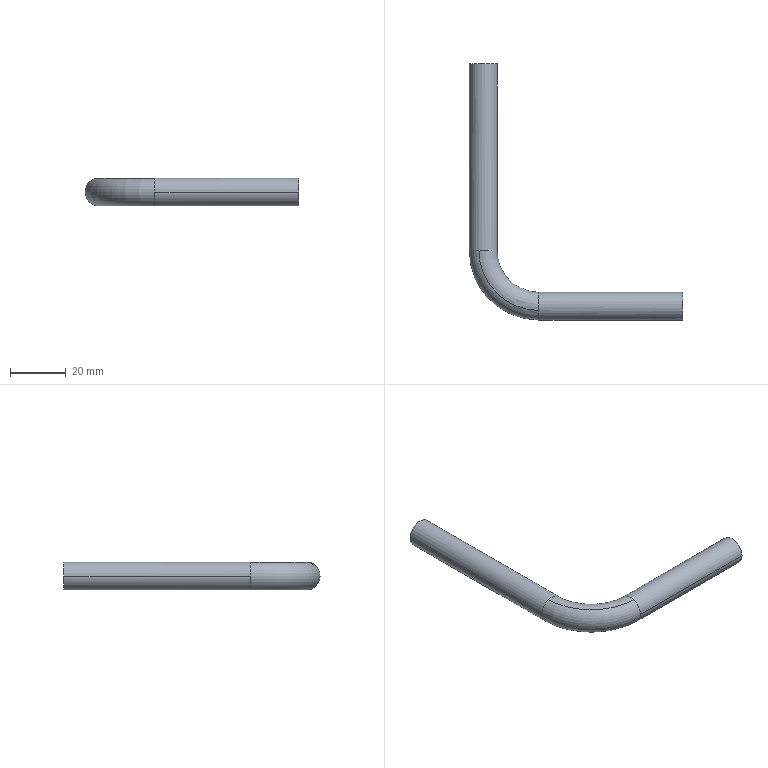Part | 1 solid | 8 faces | box 76.634 x 92 x 10 mm | volume 11785 mm3 | cylinder 4 | plane 2 | torus 2 | commonest cylinder face diameters 10 x4
STEP:
#1=CARTESIAN_POINT('',(0.,0.,0.));
#2=DIRECTION('',(0.,0.,1.));
#3=DIRECTION('',(1.,0.,0.));
#4=AXIS2_PLACEMENT_3D('',#1,#2,#3);
#5=CARTESIAN_POINT('',(-70.758,421.551,-68.051));
#6=VERTEX_POINT('',#5);
#7=CARTESIAN_POINT('',(-70.758,488.551,-68.051));
#8=VERTEX_POINT('',#7);
#9=CARTESIAN_POINT('',(-70.758,421.551,-68.051));
#10=DIRECTION('',(0.,1.,0.));
#11=VECTOR('',#10,1.);
#12=LINE('',#9,#11);
#13=CARTESIAN_POINT('',(-75.758,421.551,-68.051));
#14=DIRECTION('',(0.,1.,0.));
#15=DIRECTION('',(0.,0.,1.));
#16=AXIS2_PLACEMENT_3D('',#13,#14,#15);
#17=CYLINDRICAL_SURFACE('',#16,5.);
#18=CARTESIAN_POINT('',(1.571,0.));
#19=DIRECTION('',(0.,1.));
#20=VECTOR('',#19,1.);
#21=LINE('',#18,#20);
#22=(GEOMETRIC_REPRESENTATION_CONTEXT(2)PARAMETRIC_REPRESENTATION_CONTEXT()REPRESENTATION_CONTEXT('',''));
#23=DEFINITIONAL_REPRESENTATION('',(#21),#22);
#24=PCURVE('',#17,#23);
#25=CARTESIAN_POINT('',(-75.758,421.551,-68.051));
#26=DIRECTION('',(0.,1.,0.));
#27=DIRECTION('',(0.,0.,-1.));
#28=AXIS2_PLACEMENT_3D('',#25,#26,#27);
#29=CYLINDRICAL_SURFACE('',#28,5.);
#30=CARTESIAN_POINT('',(4.712,0.));
#31=DIRECTION('',(0.,1.));
#32=VECTOR('',#31,1.);
#33=LINE('',#30,#32);
#34=(GEOMETRIC_REPRESENTATION_CONTEXT(2)PARAMETRIC_REPRESENTATION_CONTEXT()REPRESENTATION_CONTEXT('',''));
#35=DEFINITIONAL_REPRESENTATION('',(#33),#34);
#36=PCURVE('',#29,#35);
#37=SURFACE_CURVE('',#12,(#24,#36),.PCURVE_S1.);
#38=EDGE_CURVE('',#6,#8,#37,.T.);
#39=ORIENTED_EDGE('',*,*,#38,.F.);
#40=CARTESIAN_POINT('',(-74.213,421.551,-72.807));
#41=VERTEX_POINT('',#40);
#42=CARTESIAN_POINT('',(-75.758,421.551,-68.051));
#43=DIRECTION('',(0.,1.,0.));
#44=DIRECTION('',(-1.,0.,0.));
#45=AXIS2_PLACEMENT_3D('',#42,#43,#44);
#46=CIRCLE('',#45,5.);
#47=CARTESIAN_POINT('',(-1.571,0.));
#48=DIRECTION('',(1.,0.));
#49=VECTOR('',#48,1.);
#50=LINE('',#47,#49);
#51=(GEOMETRIC_REPRESENTATION_CONTEXT(2)PARAMETRIC_REPRESENTATION_CONTEXT()REPRESENTATION_CONTEXT('',''));
#52=DEFINITIONAL_REPRESENTATION('',(#50),#51);
#53=PCURVE('',#17,#52);
#54=CARTESIAN_POINT('',(-55.758,421.551,-68.051));
#55=DIRECTION('',(0.,0.,1.));
#56=DIRECTION('',(0.7071,0.7071,0.));
#57=AXIS2_PLACEMENT_3D('',#54,#55,#56);
#58=TOROIDAL_SURFACE('',#57,20.,5.);
#59=CARTESIAN_POINT('',(2.356,0.));
#60=DIRECTION('',(0.,1.));
#61=VECTOR('',#60,1.);
#62=LINE('',#59,#61);
#63=(GEOMETRIC_REPRESENTATION_CONTEXT(2)PARAMETRIC_REPRESENTATION_CONTEXT()REPRESENTATION_CONTEXT('',''));
#64=DEFINITIONAL_REPRESENTATION('',(#62),#63);
#65=PCURVE('',#58,#64);
#66=SURFACE_CURVE('',#46,(#53,#65),.PCURVE_S1.);
#67=EDGE_CURVE('',#6,#41,#66,.T.);
#68=ORIENTED_EDGE('',*,*,#67,.T.);
#69=CARTESIAN_POINT('',(-80.758,421.551,-68.051));
#70=VERTEX_POINT('',#69);
#71=CARTESIAN_POINT('',(-75.758,421.551,-68.051));
#72=DIRECTION('',(0.,1.,0.));
#73=DIRECTION('',(-1.,0.,0.));
#74=AXIS2_PLACEMENT_3D('',#71,#72,#73);
#75=CIRCLE('',#74,5.);
#76=CARTESIAN_POINT('',(-1.571,0.));
#77=DIRECTION('',(1.,0.));
#78=VECTOR('',#77,1.);
#79=LINE('',#76,#78);
#80=(GEOMETRIC_REPRESENTATION_CONTEXT(2)PARAMETRIC_REPRESENTATION_CONTEXT()REPRESENTATION_CONTEXT('',''));
#81=DEFINITIONAL_REPRESENTATION('',(#79),#80);
#82=PCURVE('',#17,#81);
#83=CARTESIAN_POINT('',(-55.758,421.551,-68.051));
#84=DIRECTION('',(0.,0.,1.));
#85=DIRECTION('',(0.7071,0.7071,0.));
#86=AXIS2_PLACEMENT_3D('',#83,#84,#85);
#87=TOROIDAL_SURFACE('',#86,20.,5.);
#88=CARTESIAN_POINT('',(2.356,0.));
#89=DIRECTION('',(0.,1.));
#90=VECTOR('',#89,1.);
#91=LINE('',#88,#90);
#92=(GEOMETRIC_REPRESENTATION_CONTEXT(2)PARAMETRIC_REPRESENTATION_CONTEXT()REPRESENTATION_CONTEXT('',''));
#93=DEFINITIONAL_REPRESENTATION('',(#91),#92);
#94=PCURVE('',#87,#93);
#95=SURFACE_CURVE('',#75,(#82,#94),.PCURVE_S1.);
#96=EDGE_CURVE('',#41,#70,#95,.T.);
#97=ORIENTED_EDGE('',*,*,#96,.T.);
#98=CARTESIAN_POINT('',(-80.758,488.551,-68.051));
#99=VERTEX_POINT('',#98);
#100=CARTESIAN_POINT('',(-80.758,421.551,-68.051));
#101=DIRECTION('',(0.,1.,0.));
#102=VECTOR('',#101,1.);
#103=LINE('',#100,#102);
#104=CARTESIAN_POINT('',(4.712,0.));
#105=DIRECTION('',(0.,1.));
#106=VECTOR('',#105,1.);
#107=LINE('',#104,#106);
#108=(GEOMETRIC_REPRESENTATION_CONTEXT(2)PARAMETRIC_REPRESENTATION_CONTEXT()REPRESENTATION_CONTEXT('',''));
#109=DEFINITIONAL_REPRESENTATION('',(#107),#108);
#110=PCURVE('',#17,#109);
#111=CARTESIAN_POINT('',(1.571,0.));
#112=DIRECTION('',(0.,1.));
#113=VECTOR('',#112,1.);
#114=LINE('',#111,#113);
#115=(GEOMETRIC_REPRESENTATION_CONTEXT(2)PARAMETRIC_REPRESENTATION_CONTEXT()REPRESENTATION_CONTEXT('',''));
#116=DEFINITIONAL_REPRESENTATION('',(#114),#115);
#117=PCURVE('',#29,#116);
#118=SURFACE_CURVE('',#103,(#110,#117),.PCURVE_S1.);
#119=EDGE_CURVE('',#70,#99,#118,.T.);
#120=ORIENTED_EDGE('',*,*,#119,.T.);
#121=CARTESIAN_POINT('',(-75.758,488.551,-68.051));
#122=DIRECTION('',(0.,1.,0.));
#123=DIRECTION('',(-1.,0.,0.));
#124=AXIS2_PLACEMENT_3D('',#121,#122,#123);
#125=CIRCLE('',#124,5.);
#126=CARTESIAN_POINT('',(-1.571,67.));
#127=DIRECTION('',(1.,0.));
#128=VECTOR('',#127,1.);
#129=LINE('',#126,#128);
#130=(GEOMETRIC_REPRESENTATION_CONTEXT(2)PARAMETRIC_REPRESENTATION_CONTEXT()REPRESENTATION_CONTEXT('',''));
#131=DEFINITIONAL_REPRESENTATION('',(#129),#130);
#132=PCURVE('',#17,#131);
#133=CARTESIAN_POINT('',(-75.758,488.551,-68.051));
#134=DIRECTION('',(0.,1.,0.));
#135=DIRECTION('',(-1.,0.,0.));
#136=AXIS2_PLACEMENT_3D('',#133,#134,#135);
#137=PLANE('',#136);
#138=CARTESIAN_POINT('',(0.,0.));
#139=DIRECTION('',(1.,0.));
#140=AXIS2_PLACEMENT_2D('',#138,#139);
#141=CIRCLE('',#140,5.);
#142=(GEOMETRIC_REPRESENTATION_CONTEXT(2)PARAMETRIC_REPRESENTATION_CONTEXT()REPRESENTATION_CONTEXT('',''));
#143=DEFINITIONAL_REPRESENTATION('',(#141),#142);
#144=PCURVE('',#137,#143);
#145=SURFACE_CURVE('',#125,(#132,#144),.PCURVE_S1.);
#146=EDGE_CURVE('',#8,#99,#145,.T.);
#147=ORIENTED_EDGE('',*,*,#146,.F.);
#148=EDGE_LOOP('',(#39,#68,#97,#120,#147));
#149=FACE_BOUND('',#148,.T.);
#150=ADVANCED_FACE('',(#149),#17,.T.);
#151=CARTESIAN_POINT('',(-75.758,488.551,-68.051));
#152=DIRECTION('',(0.,1.,0.));
#153=DIRECTION('',(-1.,0.,0.));
#154=AXIS2_PLACEMENT_3D('',#151,#152,#153);
#155=CIRCLE('',#154,5.);
#156=CARTESIAN_POINT('',(0.,0.));
#157=DIRECTION('',(1.,0.));
#158=AXIS2_PLACEMENT_2D('',#156,#157);
#159=CIRCLE('',#158,5.);
#160=(GEOMETRIC_REPRESENTATION_CONTEXT(2)PARAMETRIC_REPRESENTATION_CONTEXT()REPRESENTATION_CONTEXT('',''));
#161=DEFINITIONAL_REPRESENTATION('',(#159),#160);
#162=PCURVE('',#137,#161);
#163=CARTESIAN_POINT('',(1.571,67.));
#164=DIRECTION('',(1.,0.));
#165=VECTOR('',#164,1.);
#166=LINE('',#163,#165);
#167=(GEOMETRIC_REPRESENTATION_CONTEXT(2)PARAMETRIC_REPRESENTATION_CONTEXT()REPRESENTATION_CONTEXT('',''));
#168=DEFINITIONAL_REPRESENTATION('',(#166),#167);
#169=PCURVE('',#29,#168);
#170=SURFACE_CURVE('',#155,(#162,#169),.PCURVE_S1.);
#171=EDGE_CURVE('',#99,#8,#170,.T.);
#172=ORIENTED_EDGE('',*,*,#171,.T.);
#173=ORIENTED_EDGE('',*,*,#146,.T.);
#174=EDGE_LOOP('',(#172,#173));
#175=FACE_BOUND('',#174,.T.);
#176=ADVANCED_FACE('',(#175),#137,.T.);
#177=CARTESIAN_POINT('',(-55.758,403.096,-72.807));
#178=VERTEX_POINT('',#177);
#179=CARTESIAN_POINT('',(-55.758,421.551,-72.807));
#180=DIRECTION('',(0.,0.,1.));
#181=DIRECTION('',(-1.,0.,0.));
#182=AXIS2_PLACEMENT_3D('',#179,#180,#181);
#183=CIRCLE('',#182,18.455);
#184=CARTESIAN_POINT('',(2.356,4.398));
#185=DIRECTION('',(1.,0.));
#186=VECTOR('',#185,1.);
#187=LINE('',#184,#186);
#188=(GEOMETRIC_REPRESENTATION_CONTEXT(2)PARAMETRIC_REPRESENTATION_CONTEXT()REPRESENTATION_CONTEXT('',''));
#189=DEFINITIONAL_REPRESENTATION('',(#187),#188);
#190=PCURVE('',#58,#189);
#191=CARTESIAN_POINT('',(2.356,4.398));
#192=DIRECTION('',(1.,0.));
#193=VECTOR('',#192,1.);
#194=LINE('',#191,#193);
#195=(GEOMETRIC_REPRESENTATION_CONTEXT(2)PARAMETRIC_REPRESENTATION_CONTEXT()REPRESENTATION_CONTEXT('',''));
#196=DEFINITIONAL_REPRESENTATION('',(#194),#195);
#197=PCURVE('',#87,#196);
#198=SURFACE_CURVE('',#183,(#190,#197),.PCURVE_S1.);
#199=EDGE_CURVE('',#41,#178,#198,.T.);
#200=ORIENTED_EDGE('',*,*,#199,.F.);
#201=ORIENTED_EDGE('',*,*,#67,.F.);
#202=CARTESIAN_POINT('',(-77.304,421.551,-63.296));
#203=VERTEX_POINT('',#202);
#204=CARTESIAN_POINT('',(-75.758,421.551,-68.051));
#205=DIRECTION('',(0.,1.,0.));
#206=DIRECTION('',(-1.,0.,0.));
#207=AXIS2_PLACEMENT_3D('',#204,#205,#206);
#208=CIRCLE('',#207,5.);
#209=CARTESIAN_POINT('',(2.356,0.));
#210=DIRECTION('',(0.,1.));
#211=VECTOR('',#210,1.);
#212=LINE('',#209,#211);
#213=(GEOMETRIC_REPRESENTATION_CONTEXT(2)PARAMETRIC_REPRESENTATION_CONTEXT()REPRESENTATION_CONTEXT('',''));
#214=DEFINITIONAL_REPRESENTATION('',(#212),#213);
#215=PCURVE('',#58,#214);
#216=CARTESIAN_POINT('',(1.571,0.));
#217=DIRECTION('',(1.,0.));
#218=VECTOR('',#217,1.);
#219=LINE('',#216,#218);
#220=(GEOMETRIC_REPRESENTATION_CONTEXT(2)PARAMETRIC_REPRESENTATION_CONTEXT()REPRESENTATION_CONTEXT('',''));
#221=DEFINITIONAL_REPRESENTATION('',(#219),#220);
#222=PCURVE('',#29,#221);
#223=SURFACE_CURVE('',#208,(#215,#222),.PCURVE_S1.);
#224=EDGE_CURVE('',#203,#6,#223,.T.);
#225=ORIENTED_EDGE('',*,*,#224,.F.);
#226=CARTESIAN_POINT('',(-55.758,400.006,-63.296));
#227=VERTEX_POINT('',#226);
#228=CARTESIAN_POINT('',(-55.758,421.551,-63.296));
#229=DIRECTION('',(0.,0.,1.));
#230=DIRECTION('',(-1.,0.,0.));
#231=AXIS2_PLACEMENT_3D('',#228,#229,#230);
#232=CIRCLE('',#231,21.545);
#233=CARTESIAN_POINT('',(2.356,1.257));
#234=DIRECTION('',(1.,0.));
#235=VECTOR('',#234,1.);
#236=LINE('',#233,#235);
#237=(GEOMETRIC_REPRESENTATION_CONTEXT(2)PARAMETRIC_REPRESENTATION_CONTEXT()REPRESENTATION_CONTEXT('',''));
#238=DEFINITIONAL_REPRESENTATION('',(#236),#237);
#239=PCURVE('',#58,#238);
#240=CARTESIAN_POINT('',(2.356,7.54));
#241=DIRECTION('',(1.,0.));
#242=VECTOR('',#241,1.);
#243=LINE('',#240,#242);
#244=(GEOMETRIC_REPRESENTATION_CONTEXT(2)PARAMETRIC_REPRESENTATION_CONTEXT()REPRESENTATION_CONTEXT('',''));
#245=DEFINITIONAL_REPRESENTATION('',(#243),#244);
#246=PCURVE('',#87,#245);
#247=SURFACE_CURVE('',#232,(#239,#246),.PCURVE_S1.);
#248=EDGE_CURVE('',#203,#227,#247,.T.);
#249=ORIENTED_EDGE('',*,*,#248,.T.);
#250=CARTESIAN_POINT('',(-55.758,406.551,-68.051));
#251=VERTEX_POINT('',#250);
#252=CARTESIAN_POINT('',(-55.758,401.551,-68.051));
#253=DIRECTION('',(-1.,0.,0.));
#254=DIRECTION('',(0.,-1.,0.));
#255=AXIS2_PLACEMENT_3D('',#252,#253,#254);
#256=CIRCLE('',#255,5.);
#257=CARTESIAN_POINT('',(3.927,0.));
#258=DIRECTION('',(0.,1.));
#259=VECTOR('',#258,1.);
#260=LINE('',#257,#259);
#261=(GEOMETRIC_REPRESENTATION_CONTEXT(2)PARAMETRIC_REPRESENTATION_CONTEXT()REPRESENTATION_CONTEXT('',''));
#262=DEFINITIONAL_REPRESENTATION('',(#260),#261);
#263=PCURVE('',#58,#262);
#264=CARTESIAN_POINT('',(-55.758,401.551,-68.051));
#265=DIRECTION('',(1.,0.,0.));
#266=DIRECTION('',(0.,0.,-1.));
#267=AXIS2_PLACEMENT_3D('',#264,#265,#266);
#268=CYLINDRICAL_SURFACE('',#267,5.);
#269=CARTESIAN_POINT('',(4.712,0.));
#270=DIRECTION('',(-1.,0.));
#271=VECTOR('',#270,1.);
#272=LINE('',#269,#271);
#273=(GEOMETRIC_REPRESENTATION_CONTEXT(2)PARAMETRIC_REPRESENTATION_CONTEXT()REPRESENTATION_CONTEXT('',''));
#274=DEFINITIONAL_REPRESENTATION('',(#272),#273);
#275=PCURVE('',#268,#274);
#276=SURFACE_CURVE('',#256,(#263,#275),.PCURVE_S1.);
#277=EDGE_CURVE('',#227,#251,#276,.T.);
#278=ORIENTED_EDGE('',*,*,#277,.T.);
#279=CARTESIAN_POINT('',(-55.758,401.551,-68.051));
#280=DIRECTION('',(-1.,0.,0.));
#281=DIRECTION('',(0.,-1.,0.));
#282=AXIS2_PLACEMENT_3D('',#279,#280,#281);
#283=CIRCLE('',#282,5.);
#284=CARTESIAN_POINT('',(3.927,0.));
#285=DIRECTION('',(0.,1.));
#286=VECTOR('',#285,1.);
#287=LINE('',#284,#286);
#288=(GEOMETRIC_REPRESENTATION_CONTEXT(2)PARAMETRIC_REPRESENTATION_CONTEXT()REPRESENTATION_CONTEXT('',''));
#289=DEFINITIONAL_REPRESENTATION('',(#287),#288);
#290=PCURVE('',#58,#289);
#291=CARTESIAN_POINT('',(-55.758,401.551,-68.051));
#292=DIRECTION('',(1.,0.,0.));
#293=DIRECTION('',(0.,0.,1.));
#294=AXIS2_PLACEMENT_3D('',#291,#292,#293);
#295=CYLINDRICAL_SURFACE('',#294,5.);
#296=CARTESIAN_POINT('',(7.854,0.));
#297=DIRECTION('',(-1.,0.));
#298=VECTOR('',#297,1.);
#299=LINE('',#296,#298);
#300=(GEOMETRIC_REPRESENTATION_CONTEXT(2)PARAMETRIC_REPRESENTATION_CONTEXT()REPRESENTATION_CONTEXT('',''));
#301=DEFINITIONAL_REPRESENTATION('',(#299),#300);
#302=PCURVE('',#295,#301);
#303=SURFACE_CURVE('',#283,(#290,#302),.PCURVE_S1.);
#304=EDGE_CURVE('',#251,#178,#303,.T.);
#305=ORIENTED_EDGE('',*,*,#304,.T.);
#306=EDGE_LOOP('',(#200,#201,#225,#249,#278,#305));
#307=FACE_BOUND('',#306,.T.);
#308=ADVANCED_FACE('',(#307),#58,.T.);
#309=CARTESIAN_POINT('',(-55.758,396.551,-68.051));
#310=VERTEX_POINT('',#309);
#311=CARTESIAN_POINT('',(-4.124,396.551,-68.051));
#312=VERTEX_POINT('',#311);
#313=CARTESIAN_POINT('',(-55.758,396.551,-68.051));
#314=DIRECTION('',(1.,0.,0.));
#315=VECTOR('',#314,1.);
#316=LINE('',#313,#315);
#317=CARTESIAN_POINT('',(1.571,0.));
#318=DIRECTION('',(0.,1.));
#319=VECTOR('',#318,1.);
#320=LINE('',#317,#319);
#321=(GEOMETRIC_REPRESENTATION_CONTEXT(2)PARAMETRIC_REPRESENTATION_CONTEXT()REPRESENTATION_CONTEXT('',''));
#322=DEFINITIONAL_REPRESENTATION('',(#320),#321);
#323=PCURVE('',#295,#322);
#324=CARTESIAN_POINT('',(4.712,0.));
#325=DIRECTION('',(0.,1.));
#326=VECTOR('',#325,1.);
#327=LINE('',#324,#326);
#328=(GEOMETRIC_REPRESENTATION_CONTEXT(2)PARAMETRIC_REPRESENTATION_CONTEXT()REPRESENTATION_CONTEXT('',''));
#329=DEFINITIONAL_REPRESENTATION('',(#327),#328);
#330=PCURVE('',#268,#329);
#331=SURFACE_CURVE('',#316,(#323,#330),.PCURVE_S1.);
#332=EDGE_CURVE('',#310,#312,#331,.T.);
#333=ORIENTED_EDGE('',*,*,#332,.F.);
#334=CARTESIAN_POINT('',(-55.758,401.551,-68.051));
#335=DIRECTION('',(-1.,0.,0.));
#336=DIRECTION('',(0.,-1.,0.));
#337=AXIS2_PLACEMENT_3D('',#334,#335,#336);
#338=CIRCLE('',#337,5.);
#339=CARTESIAN_POINT('',(7.854,0.));
#340=DIRECTION('',(-1.,0.));
#341=VECTOR('',#340,1.);
#342=LINE('',#339,#341);
#343=(GEOMETRIC_REPRESENTATION_CONTEXT(2)PARAMETRIC_REPRESENTATION_CONTEXT()REPRESENTATION_CONTEXT('',''));
#344=DEFINITIONAL_REPRESENTATION('',(#342),#343);
#345=PCURVE('',#295,#344);
#346=CARTESIAN_POINT('',(3.927,0.));
#347=DIRECTION('',(0.,1.));
#348=VECTOR('',#347,1.);
#349=LINE('',#346,#348);
#350=(GEOMETRIC_REPRESENTATION_CONTEXT(2)PARAMETRIC_REPRESENTATION_CONTEXT()REPRESENTATION_CONTEXT('',''));
#351=DEFINITIONAL_REPRESENTATION('',(#349),#350);
#352=PCURVE('',#87,#351);
#353=SURFACE_CURVE('',#338,(#345,#352),.PCURVE_S1.);
#354=EDGE_CURVE('',#178,#310,#353,.T.);
#355=ORIENTED_EDGE('',*,*,#354,.F.);
#356=ORIENTED_EDGE('',*,*,#304,.F.);
#357=CARTESIAN_POINT('',(-4.124,406.551,-68.051));
#358=VERTEX_POINT('',#357);
#359=CARTESIAN_POINT('',(-55.758,406.551,-68.051));
#360=DIRECTION('',(1.,0.,0.));
#361=VECTOR('',#360,1.);
#362=LINE('',#359,#361);
#363=CARTESIAN_POINT('',(4.712,0.));
#364=DIRECTION('',(0.,1.));
#365=VECTOR('',#364,1.);
#366=LINE('',#363,#365);
#367=(GEOMETRIC_REPRESENTATION_CONTEXT(2)PARAMETRIC_REPRESENTATION_CONTEXT()REPRESENTATION_CONTEXT('',''));
#368=DEFINITIONAL_REPRESENTATION('',(#366),#367);
#369=PCURVE('',#295,#368);
#370=CARTESIAN_POINT('',(1.571,0.));
#371=DIRECTION('',(0.,1.));
#372=VECTOR('',#371,1.);
#373=LINE('',#370,#372);
#374=(GEOMETRIC_REPRESENTATION_CONTEXT(2)PARAMETRIC_REPRESENTATION_CONTEXT()REPRESENTATION_CONTEXT('',''));
#375=DEFINITIONAL_REPRESENTATION('',(#373),#374);
#376=PCURVE('',#268,#375);
#377=SURFACE_CURVE('',#362,(#369,#376),.PCURVE_S1.);
#378=EDGE_CURVE('',#251,#358,#377,.T.);
#379=ORIENTED_EDGE('',*,*,#378,.T.);
#380=CARTESIAN_POINT('',(-4.124,401.551,-68.051));
#381=DIRECTION('',(-1.,0.,0.));
#382=DIRECTION('',(0.,1.,0.));
#383=AXIS2_PLACEMENT_3D('',#380,#381,#382);
#384=CIRCLE('',#383,5.);
#385=CARTESIAN_POINT('',(4.712,51.634));
#386=DIRECTION('',(-1.,0.));
#387=VECTOR('',#386,1.);
#388=LINE('',#385,#387);
#389=(GEOMETRIC_REPRESENTATION_CONTEXT(2)PARAMETRIC_REPRESENTATION_CONTEXT()REPRESENTATION_CONTEXT('',''));
#390=DEFINITIONAL_REPRESENTATION('',(#388),#389);
#391=PCURVE('',#295,#390);
#392=CARTESIAN_POINT('',(-4.124,401.551,-68.051));
#393=DIRECTION('',(-1.,0.,0.));
#394=DIRECTION('',(0.,-1.,0.));
#395=AXIS2_PLACEMENT_3D('',#392,#393,#394);
#396=PLANE('',#395);
#397=CARTESIAN_POINT('',(0.,0.));
#398=DIRECTION('',(-1.,0.));
#399=AXIS2_PLACEMENT_2D('',#397,#398);
#400=CIRCLE('',#399,5.);
#401=(GEOMETRIC_REPRESENTATION_CONTEXT(2)PARAMETRIC_REPRESENTATION_CONTEXT()REPRESENTATION_CONTEXT('',''));
#402=DEFINITIONAL_REPRESENTATION('',(#400),#401);
#403=PCURVE('',#396,#402);
#404=SURFACE_CURVE('',#384,(#391,#403),.PCURVE_S1.);
#405=EDGE_CURVE('',#358,#312,#404,.T.);
#406=ORIENTED_EDGE('',*,*,#405,.T.);
#407=EDGE_LOOP('',(#333,#355,#356,#379,#406));
#408=FACE_BOUND('',#407,.T.);
#409=ADVANCED_FACE('',(#408),#295,.T.);
#410=CARTESIAN_POINT('',(-4.124,401.551,-68.051));
#411=DIRECTION('',(-1.,0.,0.));
#412=DIRECTION('',(0.,1.,0.));
#413=AXIS2_PLACEMENT_3D('',#410,#411,#412);
#414=CIRCLE('',#413,5.);
#415=CARTESIAN_POINT('',(0.,0.));
#416=DIRECTION('',(-1.,0.));
#417=AXIS2_PLACEMENT_2D('',#415,#416);
#418=CIRCLE('',#417,5.);
#419=(GEOMETRIC_REPRESENTATION_CONTEXT(2)PARAMETRIC_REPRESENTATION_CONTEXT()REPRESENTATION_CONTEXT('',''));
#420=DEFINITIONAL_REPRESENTATION('',(#418),#419);
#421=PCURVE('',#396,#420);
#422=CARTESIAN_POINT('',(7.854,51.634));
#423=DIRECTION('',(-1.,0.));
#424=VECTOR('',#423,1.);
#425=LINE('',#422,#424);
#426=(GEOMETRIC_REPRESENTATION_CONTEXT(2)PARAMETRIC_REPRESENTATION_CONTEXT()REPRESENTATION_CONTEXT('',''));
#427=DEFINITIONAL_REPRESENTATION('',(#425),#426);
#428=PCURVE('',#268,#427);
#429=SURFACE_CURVE('',#414,(#421,#428),.PCURVE_S1.);
#430=EDGE_CURVE('',#312,#358,#429,.T.);
#431=ORIENTED_EDGE('',*,*,#430,.F.);
#432=ORIENTED_EDGE('',*,*,#405,.F.);
#433=EDGE_LOOP('',(#431,#432));
#434=FACE_BOUND('',#433,.T.);
#435=ADVANCED_FACE('',(#434),#396,.F.);
#436=ORIENTED_EDGE('',*,*,#38,.T.);
#437=ORIENTED_EDGE('',*,*,#171,.F.);
#438=ORIENTED_EDGE('',*,*,#119,.F.);
#439=CARTESIAN_POINT('',(-75.758,421.551,-68.051));
#440=DIRECTION('',(0.,1.,0.));
#441=DIRECTION('',(-1.,0.,0.));
#442=AXIS2_PLACEMENT_3D('',#439,#440,#441);
#443=CIRCLE('',#442,5.);
#444=CARTESIAN_POINT('',(1.571,0.));
#445=DIRECTION('',(1.,0.));
#446=VECTOR('',#445,1.);
#447=LINE('',#444,#446);
#448=(GEOMETRIC_REPRESENTATION_CONTEXT(2)PARAMETRIC_REPRESENTATION_CONTEXT()REPRESENTATION_CONTEXT('',''));
#449=DEFINITIONAL_REPRESENTATION('',(#447),#448);
#450=PCURVE('',#29,#449);
#451=CARTESIAN_POINT('',(2.356,6.283));
#452=DIRECTION('',(0.,1.));
#453=VECTOR('',#452,1.);
#454=LINE('',#451,#453);
#455=(GEOMETRIC_REPRESENTATION_CONTEXT(2)PARAMETRIC_REPRESENTATION_CONTEXT()REPRESENTATION_CONTEXT('',''));
#456=DEFINITIONAL_REPRESENTATION('',(#454),#455);
#457=PCURVE('',#87,#456);
#458=SURFACE_CURVE('',#443,(#450,#457),.PCURVE_S1.);
#459=EDGE_CURVE('',#70,#203,#458,.T.);
#460=ORIENTED_EDGE('',*,*,#459,.T.);
#461=ORIENTED_EDGE('',*,*,#224,.T.);
#462=EDGE_LOOP('',(#436,#437,#438,#460,#461));
#463=FACE_BOUND('',#462,.T.);
#464=ADVANCED_FACE('',(#463),#29,.T.);
#465=ORIENTED_EDGE('',*,*,#199,.T.);
#466=ORIENTED_EDGE('',*,*,#354,.T.);
#467=CARTESIAN_POINT('',(-55.758,401.551,-68.051));
#468=DIRECTION('',(-1.,0.,0.));
#469=DIRECTION('',(0.,-1.,0.));
#470=AXIS2_PLACEMENT_3D('',#467,#468,#469);
#471=CIRCLE('',#470,5.);
#472=CARTESIAN_POINT('',(3.927,6.283));
#473=DIRECTION('',(0.,1.));
#474=VECTOR('',#473,1.);
#475=LINE('',#472,#474);
#476=(GEOMETRIC_REPRESENTATION_CONTEXT(2)PARAMETRIC_REPRESENTATION_CONTEXT()REPRESENTATION_CONTEXT('',''));
#477=DEFINITIONAL_REPRESENTATION('',(#475),#476);
#478=PCURVE('',#87,#477);
#479=CARTESIAN_POINT('',(4.712,0.));
#480=DIRECTION('',(-1.,0.));
#481=VECTOR('',#480,1.);
#482=LINE('',#479,#481);
#483=(GEOMETRIC_REPRESENTATION_CONTEXT(2)PARAMETRIC_REPRESENTATION_CONTEXT()REPRESENTATION_CONTEXT('',''));
#484=DEFINITIONAL_REPRESENTATION('',(#482),#483);
#485=PCURVE('',#268,#484);
#486=SURFACE_CURVE('',#471,(#478,#485),.PCURVE_S1.);
#487=EDGE_CURVE('',#310,#227,#486,.T.);
#488=ORIENTED_EDGE('',*,*,#487,.T.);
#489=ORIENTED_EDGE('',*,*,#248,.F.);
#490=ORIENTED_EDGE('',*,*,#459,.F.);
#491=ORIENTED_EDGE('',*,*,#96,.F.);
#492=EDGE_LOOP('',(#465,#466,#488,#489,#490,#491));
#493=FACE_BOUND('',#492,.T.);
#494=ADVANCED_FACE('',(#493),#87,.T.);
#495=ORIENTED_EDGE('',*,*,#332,.T.);
#496=ORIENTED_EDGE('',*,*,#430,.T.);
#497=ORIENTED_EDGE('',*,*,#378,.F.);
#498=ORIENTED_EDGE('',*,*,#277,.F.);
#499=ORIENTED_EDGE('',*,*,#487,.F.);
#500=EDGE_LOOP('',(#495,#496,#497,#498,#499));
#501=FACE_BOUND('',#500,.T.);
#502=ADVANCED_FACE('',(#501),#268,.T.);
#503=CLOSED_SHELL('',(#150,#176,#308,#409,#435,#464,#494,#502));
#504=MANIFOLD_SOLID_BREP('',#503);
#505=(LENGTH_UNIT()NAMED_UNIT(*)SI_UNIT(.MILLI.,.METRE.));
#506=UNCERTAINTY_MEASURE_WITH_UNIT(LENGTH_MEASURE(0.0000001),#505,'','');
#507=(NAMED_UNIT(*)PLANE_ANGLE_UNIT()SI_UNIT($,.RADIAN.));
#508=(NAMED_UNIT(*)SI_UNIT($,.STERADIAN.)SOLID_ANGLE_UNIT());
#509=(GEOMETRIC_REPRESENTATION_CONTEXT(3)GLOBAL_UNCERTAINTY_ASSIGNED_CONTEXT((#506))GLOBAL_UNIT_ASSIGNED_CONTEXT((#505,#507,#508))REPRESENTATION_CONTEXT('',''));
#510=ADVANCED_BREP_SHAPE_REPRESENTATION('',(#4,#504),#509);